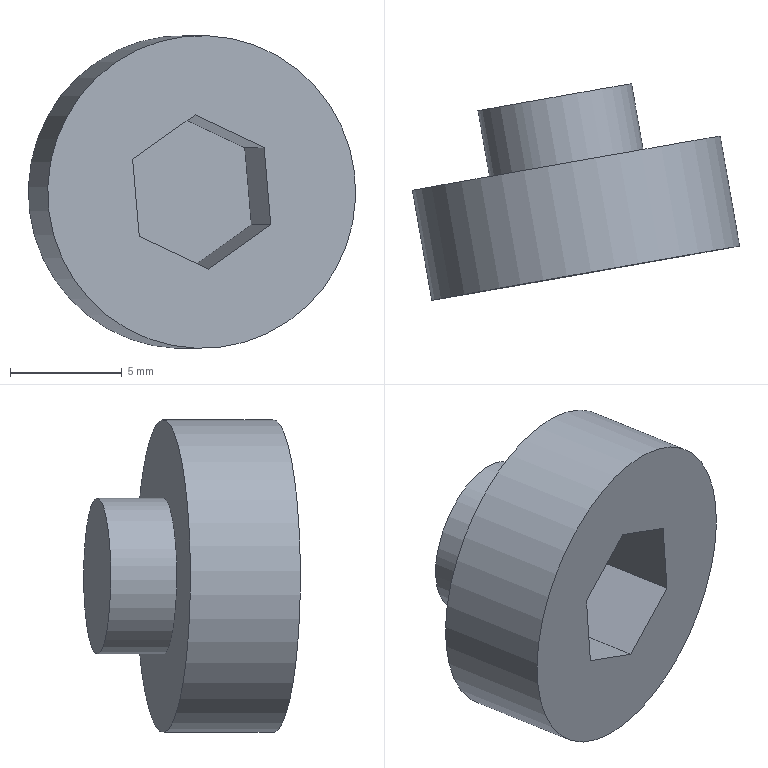Part | NX | features solid 2 | 1 solid | 12 faces | box 14.656 x 9.701 x 14 mm | volume 728.494 mm3 | plane 10 | cylinder 1 | spline 1 | commonest cylinder face diameters 14 x1
STEP:
#1=CARTESIAN_POINT('',(1661.016,567.047,-5.713));
#2=VERTEX_POINT('',#1);
#3=CARTESIAN_POINT('',(1667.494,568.189,-8.108));
#4=DIRECTION('',(-0.1736,0.9848,0.));
#5=DIRECTION('',(-0.9254,-0.1632,0.342));
#6=AXIS2_PLACEMENT_3D('',#3,#4,#5);
#7=CIRCLE('',#6,7.);
#8=EDGE_CURVE('',#2,#2,#7,.T.);
#9=ORIENTED_EDGE('',*,*,#8,.F.);
#10=EDGE_LOOP('',(#9));
#11=FACE_BOUND('',#10,.T.);
#12=CARTESIAN_POINT('',(1661.884,562.123,-5.713));
#13=VERTEX_POINT('',#12);
#14=CARTESIAN_POINT('',(1668.362,563.265,-8.108));
#15=DIRECTION('',(-0.1736,0.9848,0.));
#16=DIRECTION('',(-0.9254,-0.1632,0.342));
#17=AXIS2_PLACEMENT_3D('',#14,#15,#16);
#18=CIRCLE('',#17,7.);
#19=EDGE_CURVE('',#13,#13,#18,.T.);
#20=ORIENTED_EDGE('',*,*,#19,.T.);
#21=EDGE_LOOP('',(#20));
#22=FACE_BOUND('',#21,.T.);
#23=CARTESIAN_POINT('',(1667.494,568.189,-8.108));
#24=DIRECTION('',(0.1736,-0.9848,0.));
#25=DIRECTION('',(-0.8925,-0.1574,0.4226));
#26=AXIS2_PLACEMENT_3D('',#23,#24,#25);
#27=CYLINDRICAL_SURFACE('',#26,7.);
#28=ADVANCED_FACE('',(#11,#22),#27,.T.);
#29=CARTESIAN_POINT('',(1664.255,567.618,-6.91));
#30=VERTEX_POINT('',#29);
#31=CARTESIAN_POINT('',(1663.614,567.505,-8.698));
#32=CARTESIAN_POINT('',(1664.896,567.731,-5.123));
#33=CARTESIAN_POINT('',(1666.912,568.087,-4.168));
#34=CARTESIAN_POINT('',(1670.433,568.708,-5.469));
#35=CARTESIAN_POINT('',(1671.373,568.873,-7.517));
#36=CARTESIAN_POINT('',(1670.092,568.647,-11.092));
#37=CARTESIAN_POINT('',(1668.075,568.292,-12.047));
#38=CARTESIAN_POINT('',(1664.555,567.671,-10.746));
#39=CARTESIAN_POINT('',(1663.614,567.505,-8.698));
#40=CARTESIAN_POINT('',(1664.896,567.731,-5.123));
#41=B_SPLINE_CURVE_WITH_KNOTS('',3,(#31,#32,#33,#34,#35,#36,#37,#38,#39,#40),.UNSPECIFIED.,.T.,.F.,(2,2,2,2,2,2,2),(-0.25,0.,0.25,0.5,0.75,1.,1.25),.UNSPECIFIED.);
#42=EDGE_CURVE('',#30,#30,#41,.T.);
#43=ORIENTED_EDGE('',*,*,#42,.F.);
#44=EDGE_LOOP('',(#43));
#45=FACE_BOUND('',#44,.T.);
#46=ORIENTED_EDGE('',*,*,#8,.T.);
#47=EDGE_LOOP('',(#46));
#48=FACE_BOUND('',#47,.T.);
#49=CARTESIAN_POINT('',(1667.494,568.189,-8.108));
#50=DIRECTION('',(0.1736,-0.9848,0.));
#51=DIRECTION('',(-0.8925,-0.1574,0.4226));
#52=AXIS2_PLACEMENT_3D('',#49,#50,#51);
#53=PLANE('',#52);
#54=ADVANCED_FACE('',(#45,#48),#53,.F.);
#55=CARTESIAN_POINT('',(1668.065,563.213,-4.657));
#56=VERTEX_POINT('',#55);
#57=CARTESIAN_POINT('',(1671.157,563.758,-6.121));
#58=VERTEX_POINT('',#57);
#59=CARTESIAN_POINT('',(1668.065,563.213,-4.657));
#60=DIRECTION('',(0.8925,0.1574,-0.4226));
#61=VECTOR('',#60,1000.);
#62=LINE('',#59,#61);
#63=EDGE_CURVE('',#56,#58,#62,.T.);
#64=ORIENTED_EDGE('',*,*,#63,.T.);
#65=CARTESIAN_POINT('',(1671.454,563.81,-9.572));
#66=VERTEX_POINT('',#65);
#67=CARTESIAN_POINT('',(1671.157,563.758,-6.121));
#68=DIRECTION('',(0.08583,0.01513,-0.9962));
#69=VECTOR('',#68,1000.);
#70=LINE('',#67,#69);
#71=EDGE_CURVE('',#58,#66,#70,.T.);
#72=ORIENTED_EDGE('',*,*,#71,.T.);
#73=CARTESIAN_POINT('',(1668.659,563.318,-11.558));
#74=VERTEX_POINT('',#73);
#75=CARTESIAN_POINT('',(1671.454,563.81,-9.572));
#76=DIRECTION('',(-0.8067,-0.1422,-0.5736));
#77=VECTOR('',#76,1000.);
#78=LINE('',#75,#77);
#79=EDGE_CURVE('',#66,#74,#78,.T.);
#80=ORIENTED_EDGE('',*,*,#79,.T.);
#81=CARTESIAN_POINT('',(1665.568,562.773,-10.094));
#82=VERTEX_POINT('',#81);
#83=CARTESIAN_POINT('',(1668.659,563.318,-11.558));
#84=DIRECTION('',(-0.8925,-0.1574,0.4226));
#85=VECTOR('',#84,1000.);
#86=LINE('',#83,#85);
#87=EDGE_CURVE('',#74,#82,#86,.T.);
#88=ORIENTED_EDGE('',*,*,#87,.T.);
#89=CARTESIAN_POINT('',(1665.27,562.72,-6.644));
#90=VERTEX_POINT('',#89);
#91=CARTESIAN_POINT('',(1665.568,562.773,-10.094));
#92=DIRECTION('',(-0.08583,-0.01513,0.9962));
#93=VECTOR('',#92,1000.);
#94=LINE('',#91,#93);
#95=EDGE_CURVE('',#82,#90,#94,.T.);
#96=ORIENTED_EDGE('',*,*,#95,.T.);
#97=CARTESIAN_POINT('',(1665.27,562.72,-6.644));
#98=DIRECTION('',(0.8067,0.1422,0.5736));
#99=VECTOR('',#98,1000.);
#100=LINE('',#97,#99);
#101=EDGE_CURVE('',#90,#56,#100,.T.);
#102=ORIENTED_EDGE('',*,*,#101,.T.);
#103=EDGE_LOOP('',(#64,#72,#80,#88,#96,#102));
#104=FACE_BOUND('',#103,.T.);
#105=ORIENTED_EDGE('',*,*,#19,.F.);
#106=EDGE_LOOP('',(#105));
#107=FACE_BOUND('',#106,.T.);
#108=CARTESIAN_POINT('',(1668.362,563.265,-8.108));
#109=DIRECTION('',(0.1736,-0.9848,0.));
#110=DIRECTION('',(-0.8925,-0.1574,0.4226));
#111=AXIS2_PLACEMENT_3D('',#108,#109,#110);
#112=PLANE('',#111);
#113=ADVANCED_FACE('',(#104,#107),#112,.T.);
#114=ORIENTED_EDGE('',*,*,#63,.F.);
#115=CARTESIAN_POINT('',(1667.196,568.137,-4.657));
#116=VERTEX_POINT('',#115);
#117=CARTESIAN_POINT('',(1667.196,568.137,-4.657));
#118=DIRECTION('',(0.1736,-0.9848,0.));
#119=VECTOR('',#118,1000.);
#120=LINE('',#117,#119);
#121=EDGE_CURVE('',#116,#56,#120,.T.);
#122=ORIENTED_EDGE('',*,*,#121,.F.);
#123=CARTESIAN_POINT('',(1670.288,568.682,-6.121));
#124=VERTEX_POINT('',#123);
#125=CARTESIAN_POINT('',(1667.196,568.137,-4.657));
#126=DIRECTION('',(0.8925,0.1574,-0.4226));
#127=VECTOR('',#126,1000.);
#128=LINE('',#125,#127);
#129=EDGE_CURVE('',#116,#124,#128,.T.);
#130=ORIENTED_EDGE('',*,*,#129,.T.);
#131=CARTESIAN_POINT('',(1670.288,568.682,-6.121));
#132=DIRECTION('',(0.1736,-0.9848,0.));
#133=VECTOR('',#132,1000.);
#134=LINE('',#131,#133);
#135=EDGE_CURVE('',#124,#58,#134,.T.);
#136=ORIENTED_EDGE('',*,*,#135,.T.);
#137=EDGE_LOOP('',(#114,#122,#130,#136));
#138=FACE_BOUND('',#137,.T.);
#139=CARTESIAN_POINT('',(1667.196,568.137,-4.657));
#140=DIRECTION('',(0.4162,0.07339,0.9063));
#141=DIRECTION('',(0.1736,-0.9848,0.));
#142=AXIS2_PLACEMENT_3D('',#139,#140,#141);
#143=PLANE('',#142);
#144=ADVANCED_FACE('',(#138),#143,.F.);
#145=ORIENTED_EDGE('',*,*,#71,.F.);
#146=ORIENTED_EDGE('',*,*,#135,.F.);
#147=CARTESIAN_POINT('',(1670.586,568.735,-9.572));
#148=VERTEX_POINT('',#147);
#149=CARTESIAN_POINT('',(1670.288,568.682,-6.121));
#150=DIRECTION('',(0.08583,0.01513,-0.9962));
#151=VECTOR('',#150,1000.);
#152=LINE('',#149,#151);
#153=EDGE_CURVE('',#124,#148,#152,.T.);
#154=ORIENTED_EDGE('',*,*,#153,.T.);
#155=CARTESIAN_POINT('',(1670.586,568.735,-9.572));
#156=DIRECTION('',(0.1736,-0.9848,0.));
#157=VECTOR('',#156,1000.);
#158=LINE('',#155,#157);
#159=EDGE_CURVE('',#148,#66,#158,.T.);
#160=ORIENTED_EDGE('',*,*,#159,.T.);
#161=EDGE_LOOP('',(#145,#146,#154,#160));
#162=FACE_BOUND('',#161,.T.);
#163=CARTESIAN_POINT('',(1670.288,568.682,-6.121));
#164=DIRECTION('',(0.9811,0.173,0.08716));
#165=DIRECTION('',(0.08583,0.01513,-0.9962));
#166=AXIS2_PLACEMENT_3D('',#163,#164,#165);
#167=PLANE('',#166);
#168=ADVANCED_FACE('',(#162),#167,.F.);
#169=ORIENTED_EDGE('',*,*,#79,.F.);
#170=ORIENTED_EDGE('',*,*,#159,.F.);
#171=CARTESIAN_POINT('',(1667.791,568.242,-11.558));
#172=VERTEX_POINT('',#171);
#173=CARTESIAN_POINT('',(1670.586,568.735,-9.572));
#174=DIRECTION('',(-0.8067,-0.1422,-0.5736));
#175=VECTOR('',#174,1000.);
#176=LINE('',#173,#175);
#177=EDGE_CURVE('',#148,#172,#176,.T.);
#178=ORIENTED_EDGE('',*,*,#177,.T.);
#179=CARTESIAN_POINT('',(1667.791,568.242,-11.558));
#180=DIRECTION('',(0.1736,-0.9848,0.));
#181=VECTOR('',#180,1000.);
#182=LINE('',#179,#181);
#183=EDGE_CURVE('',#172,#74,#182,.T.);
#184=ORIENTED_EDGE('',*,*,#183,.T.);
#185=EDGE_LOOP('',(#169,#170,#178,#184));
#186=FACE_BOUND('',#185,.T.);
#187=CARTESIAN_POINT('',(1670.586,568.735,-9.572));
#188=DIRECTION('',(0.5649,0.0996,-0.8192));
#189=DIRECTION('',(-0.8067,-0.1422,-0.5736));
#190=AXIS2_PLACEMENT_3D('',#187,#188,#189);
#191=PLANE('',#190);
#192=ADVANCED_FACE('',(#186),#191,.F.);
#193=ORIENTED_EDGE('',*,*,#87,.F.);
#194=ORIENTED_EDGE('',*,*,#183,.F.);
#195=CARTESIAN_POINT('',(1664.699,567.697,-10.094));
#196=VERTEX_POINT('',#195);
#197=CARTESIAN_POINT('',(1667.791,568.242,-11.558));
#198=DIRECTION('',(-0.8925,-0.1574,0.4226));
#199=VECTOR('',#198,1000.);
#200=LINE('',#197,#199);
#201=EDGE_CURVE('',#172,#196,#200,.T.);
#202=ORIENTED_EDGE('',*,*,#201,.T.);
#203=CARTESIAN_POINT('',(1664.699,567.697,-10.094));
#204=DIRECTION('',(0.1736,-0.9848,0.));
#205=VECTOR('',#204,1000.);
#206=LINE('',#203,#205);
#207=EDGE_CURVE('',#196,#82,#206,.T.);
#208=ORIENTED_EDGE('',*,*,#207,.T.);
#209=EDGE_LOOP('',(#193,#194,#202,#208));
#210=FACE_BOUND('',#209,.T.);
#211=CARTESIAN_POINT('',(1667.791,568.242,-11.558));
#212=DIRECTION('',(-0.4162,-0.07339,-0.9063));
#213=DIRECTION('',(-0.1736,0.9848,0.));
#214=AXIS2_PLACEMENT_3D('',#211,#212,#213);
#215=PLANE('',#214);
#216=ADVANCED_FACE('',(#210),#215,.F.);
#217=ORIENTED_EDGE('',*,*,#95,.F.);
#218=ORIENTED_EDGE('',*,*,#207,.F.);
#219=CARTESIAN_POINT('',(1664.402,567.644,-6.644));
#220=VERTEX_POINT('',#219);
#221=CARTESIAN_POINT('',(1664.699,567.697,-10.094));
#222=DIRECTION('',(-0.08583,-0.01513,0.9962));
#223=VECTOR('',#222,1000.);
#224=LINE('',#221,#223);
#225=EDGE_CURVE('',#196,#220,#224,.T.);
#226=ORIENTED_EDGE('',*,*,#225,.T.);
#227=CARTESIAN_POINT('',(1664.402,567.644,-6.644));
#228=DIRECTION('',(0.1736,-0.9848,0.));
#229=VECTOR('',#228,1000.);
#230=LINE('',#227,#229);
#231=EDGE_CURVE('',#220,#90,#230,.T.);
#232=ORIENTED_EDGE('',*,*,#231,.T.);
#233=EDGE_LOOP('',(#217,#218,#226,#232));
#234=FACE_BOUND('',#233,.T.);
#235=CARTESIAN_POINT('',(1664.699,567.697,-10.094));
#236=DIRECTION('',(-0.9811,-0.173,-0.08716));
#237=DIRECTION('',(-0.08583,-0.01513,0.9962));
#238=AXIS2_PLACEMENT_3D('',#235,#236,#237);
#239=PLANE('',#238);
#240=ADVANCED_FACE('',(#234),#239,.F.);
#241=ORIENTED_EDGE('',*,*,#101,.F.);
#242=ORIENTED_EDGE('',*,*,#231,.F.);
#243=CARTESIAN_POINT('',(1664.402,567.644,-6.644));
#244=DIRECTION('',(0.8067,0.1422,0.5736));
#245=VECTOR('',#244,1000.);
#246=LINE('',#243,#245);
#247=EDGE_CURVE('',#220,#116,#246,.T.);
#248=ORIENTED_EDGE('',*,*,#247,.T.);
#249=ORIENTED_EDGE('',*,*,#121,.T.);
#250=EDGE_LOOP('',(#241,#242,#248,#249));
#251=FACE_BOUND('',#250,.T.);
#252=CARTESIAN_POINT('',(1664.402,567.644,-6.644));
#253=DIRECTION('',(-0.5649,-0.0996,0.8192));
#254=DIRECTION('',(0.8067,0.1422,0.5736));
#255=AXIS2_PLACEMENT_3D('',#252,#253,#254);
#256=PLANE('',#255);
#257=ADVANCED_FACE('',(#251),#256,.F.);
#258=ORIENTED_EDGE('',*,*,#247,.F.);
#259=ORIENTED_EDGE('',*,*,#225,.F.);
#260=ORIENTED_EDGE('',*,*,#201,.F.);
#261=ORIENTED_EDGE('',*,*,#177,.F.);
#262=ORIENTED_EDGE('',*,*,#153,.F.);
#263=ORIENTED_EDGE('',*,*,#129,.F.);
#264=EDGE_LOOP('',(#258,#259,#260,#261,#262,#263));
#265=FACE_BOUND('',#264,.T.);
#266=CARTESIAN_POINT('',(1670.733,568.76,-9.305));
#267=DIRECTION('',(-0.1736,0.9848,0.));
#268=DIRECTION('',(0.8925,0.1574,-0.4226));
#269=AXIS2_PLACEMENT_3D('',#266,#267,#268);
#270=PLANE('',#269);
#271=ADVANCED_FACE('',(#265),#270,.F.);
#272=CARTESIAN_POINT('',(1663.734,570.573,-6.91));
#273=VERTEX_POINT('',#272);
#274=CARTESIAN_POINT('',(1663.093,570.46,-8.698));
#275=CARTESIAN_POINT('',(1664.375,570.686,-5.123));
#276=CARTESIAN_POINT('',(1666.391,571.041,-4.168));
#277=CARTESIAN_POINT('',(1669.912,571.662,-5.469));
#278=CARTESIAN_POINT('',(1670.852,571.828,-7.517));
#279=CARTESIAN_POINT('',(1669.571,571.602,-11.092));
#280=CARTESIAN_POINT('',(1667.554,571.246,-12.047));
#281=CARTESIAN_POINT('',(1664.034,570.625,-10.746));
#282=CARTESIAN_POINT('',(1663.093,570.46,-8.698));
#283=CARTESIAN_POINT('',(1664.375,570.686,-5.123));
#284=B_SPLINE_CURVE_WITH_KNOTS('',3,(#274,#275,#276,#277,#278,#279,#280,#281,#282,#283),.UNSPECIFIED.,.T.,.F.,(2,2,2,2,2,2,2),(-0.25,0.,0.25,0.5,0.75,1.,1.25),.UNSPECIFIED.);
#285=EDGE_CURVE('',#273,#273,#284,.T.);
#286=ORIENTED_EDGE('',*,*,#285,.F.);
#287=EDGE_LOOP('',(#286));
#288=FACE_BOUND('',#287,.T.);
#289=ORIENTED_EDGE('',*,*,#42,.T.);
#290=EDGE_LOOP('',(#289));
#291=FACE_BOUND('',#290,.T.);
#292=CARTESIAN_POINT('',(1663.536,570.538,-9.735));
#293=CARTESIAN_POINT('',(1664.057,567.583,-9.735));
#294=CARTESIAN_POINT('',(1663.374,570.509,-6.778));
#295=CARTESIAN_POINT('',(1663.895,567.555,-6.778));
#296=CARTESIAN_POINT('',(1665.37,570.861,-4.618));
#297=CARTESIAN_POINT('',(1665.891,567.907,-4.618));
#298=CARTESIAN_POINT('',(1668.283,571.375,-4.453));
#299=CARTESIAN_POINT('',(1668.804,568.42,-4.453));
#300=CARTESIAN_POINT('',(1670.41,571.75,-6.48));
#301=CARTESIAN_POINT('',(1670.931,568.795,-6.48));
#302=CARTESIAN_POINT('',(1670.571,571.778,-9.438));
#303=CARTESIAN_POINT('',(1671.092,568.824,-9.438));
#304=CARTESIAN_POINT('',(1668.575,571.426,-11.597));
#305=CARTESIAN_POINT('',(1669.096,568.472,-11.597));
#306=CARTESIAN_POINT('',(1665.663,570.913,-11.762));
#307=CARTESIAN_POINT('',(1666.184,567.958,-11.762));
#308=CARTESIAN_POINT('',(1663.536,570.538,-9.735));
#309=CARTESIAN_POINT('',(1664.057,567.583,-9.735));
#310=CARTESIAN_POINT('',(1663.374,570.509,-6.778));
#311=CARTESIAN_POINT('',(1663.895,567.555,-6.778));
#312=CARTESIAN_POINT('',(1665.37,570.861,-4.618));
#313=CARTESIAN_POINT('',(1665.891,567.907,-4.618));
#314=B_SPLINE_SURFACE_WITH_KNOTS('',3,1,((#292,#293),(#294,#295),(#296,#297),(#298,#299),(#300,#301),(#302,#303),(#304,#305),(#306,#307),(#308,#309),(#310,#311),(#312,#313)),.SURF_OF_LINEAR_EXTRUSION.,.T.,.F.,.F.,(1,1,1,1,1,1,1,1,1,1,1,1,1,1,1),(2,2),(-0.375,-0.25,-0.125,0.,0.125,0.25,0.375,0.5,0.625,0.75,0.875,1.,1.125,1.25,1.375),(0.,1.),.UNSPECIFIED.);
#315=ADVANCED_FACE('',(#288,#291),#314,.F.);
#316=ORIENTED_EDGE('',*,*,#285,.T.);
#317=EDGE_LOOP('',(#316));
#318=FACE_BOUND('',#317,.T.);
#319=CARTESIAN_POINT('',(1670.212,571.715,-9.305));
#320=DIRECTION('',(-0.1736,0.9848,0.));
#321=DIRECTION('',(0.8925,0.1574,-0.4226));
#322=AXIS2_PLACEMENT_3D('',#319,#320,#321);
#323=PLANE('',#322);
#324=ADVANCED_FACE('',(#318),#323,.T.);
#325=CLOSED_SHELL('',(#28,#54,#113,#144,#168,#192,#216,#240,#257,#271,#315,#324));
#326=MANIFOLD_SOLID_BREP('',#325);
#327=(LENGTH_UNIT()NAMED_UNIT(*)SI_UNIT(.MILLI.,.METRE.));
#328=UNCERTAINTY_MEASURE_WITH_UNIT(LENGTH_MEASURE(0.0508),#327,'','');
#329=(NAMED_UNIT(*)PLANE_ANGLE_UNIT()SI_UNIT($,.RADIAN.));
#330=(NAMED_UNIT(*)SI_UNIT($,.STERADIAN.)SOLID_ANGLE_UNIT());
#331=(GEOMETRIC_REPRESENTATION_CONTEXT(3)GLOBAL_UNCERTAINTY_ASSIGNED_CONTEXT((#328))GLOBAL_UNIT_ASSIGNED_CONTEXT((#327,#329,#330))REPRESENTATION_CONTEXT('',''));
#332=ADVANCED_BREP_SHAPE_REPRESENTATION('',(#326),#331);